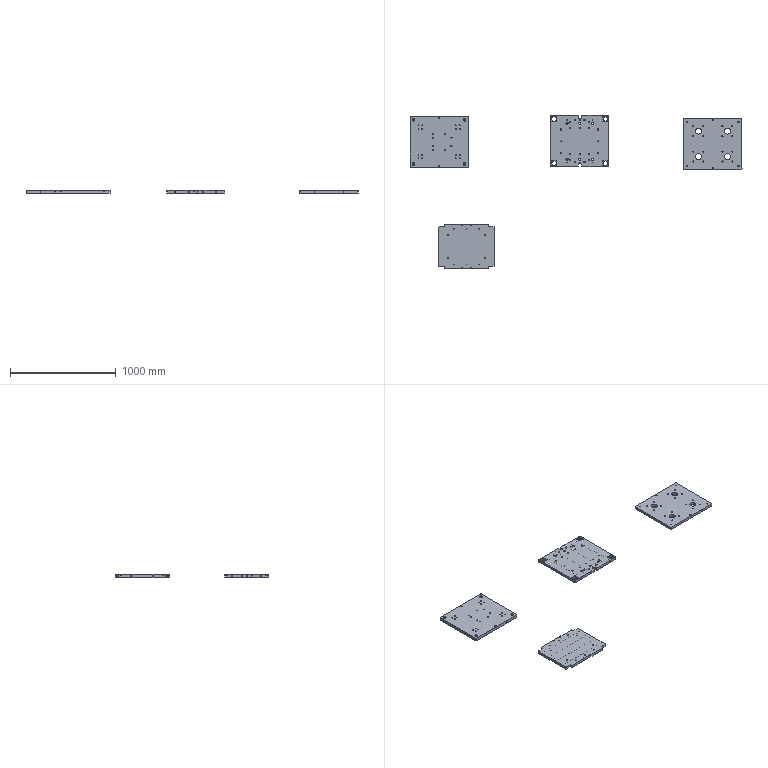NC program | Mastercam | posted with a generic post | part box 3140 x 1452 x 30 mm
Lines 4752 to 6153 of 6493, first 1239 of 1402 lines:
N7860 T7 M6
N7870 G0 G90 G17 G54 X-230.95 Y208.6 A0. S6000 M3
N7880 G43 H7 Z50. M8
N7890 Z1.2
N7900 G1 Z-.75 F600.
N7910 X-230.55 F1000.
N7920 G3 X-230.15 Y209. I0. J.4
N7930 X-242. Y220.85 I-11.85 J0.
N7940 X-253.85 Y209. I0. J-11.85
N7950 X-242. Y197.15 I11.85 J0.
N7960 X-230.15 Y209. I0. J11.85
N7970 X-230.161 Y209.5 I-11.85 J0.
N7980 X-230.56 Y209.882 I-.399 J-.017
N7990 X-230.577 Y209.883 I0. J-.399
N8000 G1 X-230.977 Y209.866
N8010 G0 Z50.
N8020 X-237.95 Y208.6
N8030 Z-11.8
N8040 G1 Z-13.75 F600.
N8050 X-237.55 F1000.
N8060 G3 X-237.15 Y209. I0. J.4
N8070 X-242. Y213.85 I-4.85 J0.
N8080 X-246.85 Y209. I0. J-4.85
N8090 X-242. Y204.15 I4.85 J0.
N8100 X-237.15 Y209. I0. J4.85
N8110 X-237.176 Y209.499 I-4.85 J0.
N8120 X-237.574 Y209.858 I-.398 J-.041
N8130 X-237.615 Y209.856 I0. J-.4
N8140 G1 X-238.013 Y209.815
N8150 G0 Z50.
N8160 X4.05 Y227.1
N8170 Z1.2
N8180 G1 Z-.75 F600.
N8190 X4.45 F1000.
N8200 G3 X4.85 Y227.5 I0. J.4
N8210 X0. Y232.35 I-4.85 J0.
N8220 X-4.85 Y227.5 I0. J-4.85
N8230 X0. Y222.65 I4.85 J0.
N8240 X4.85 Y227.5 I0. J4.85
N8250 X4.824 Y227.999 I-4.85 J0.
N8260 X4.426 Y228.358 I-.398 J-.041
N8270 X4.385 Y228.356 I0. J-.4
N8280 G1 X3.987 Y228.315
N8290 G0 Z50.
N8300 X253.05 Y208.6
N8310 Z1.2
N8320 G1 Z-.75 F600.
N8330 X253.45 F1000.
N8340 G3 X253.85 Y209. I0. J.4
N8350 X242. Y220.85 I-11.85 J0.
N8360 X230.15 Y209. I0. J-11.85
N8370 X242. Y197.15 I11.85 J0.
N8380 X253.85 Y209. I0. J11.85
N8390 X253.839 Y209.5 I-11.85 J0.
N8400 X253.44 Y209.882 I-.399 J-.017
N8410 X253.423 Y209.883 I0. J-.399
N8420 G1 X253.023 Y209.866
N8430 G0 Z50.
N8440 X246.05 Y208.6
N8450 Z-11.8
N8460 G1 Z-13.75 F600.
N8470 X246.45 F1000.
N8480 G3 X246.85 Y209. I0. J.4
N8490 X242. Y213.85 I-4.85 J0.
N8500 X237.15 Y209. I0. J-4.85
N8510 X242. Y204.15 I4.85 J0.
N8520 X246.85 Y209. I0. J4.85
N8530 X246.824 Y209.499 I-4.85 J0.
N8540 X246.426 Y209.858 I-.398 J-.041
N8550 X246.385 Y209.856 I0. J-.4
N8560 G1 X245.987 Y209.815
N8570 G0 Z50.
N8580 X197.55 Y155.6
N8590 Z1.2
N8600 G1 Z-.75 F600.
N8610 X197.95 F1000.
N8620 G3 X198.35 Y156. I0. J.4
N8630 X194.5 Y159.85 I-3.85 J0.
N8640 X190.65 Y156. I0. J-3.85
N8650 X194.5 Y152.15 I3.85 J0.
N8660 X198.35 Y156. I0. J3.85
N8670 X198.318 Y156.499 I-3.85 J0.
N8680 X197.921 Y156.847 I-.397 J-.052
N8690 X197.869 Y156.843 I0. J-.4
N8700 G1 X197.473 Y156.792
N8710 G0 Z50.
N8720 X161.55 Y155.6
N8730 Z1.2
N8740 G1 Z-.75 F600.
N8750 X161.95 F1000.
N8760 G3 X162.35 Y156. I0. J.4
N8770 X158.5 Y159.85 I-3.85 J0.
N8780 X154.65 Y156. I0. J-3.85
N8790 X158.5 Y152.15 I3.85 J0.
N8800 X162.35 Y156. I0. J3.85
N8810 X162.318 Y156.499 I-3.85 J0.
N8820 X161.921 Y156.847 I-.397 J-.052
N8830 X161.869 Y156.843 I0. J-.4
N8840 G1 X161.473 Y156.792
N8850 G0 Z50.
N8860 X161.55 Y123.6
N8870 Z1.2
N8880 G1 Z-.75 F600.
N8890 X161.95 F1000.
N8900 G3 X162.35 Y124. I0. J.4
N8910 X158.5 Y127.85 I-3.85 J0.
N8920 X154.65 Y124. I0. J-3.85
N8930 X158.5 Y120.15 I3.85 J0.
N8940 X162.35 Y124. I0. J3.85
N8950 X162.318 Y124.499 I-3.85 J0.
N8960 X161.921 Y124.847 I-.397 J-.052
N8970 X161.869 Y124.843 I0. J-.4
N8980 G1 X161.473 Y124.792
N8990 G0 Z50.
N9000 X197.55 Y123.6
N9010 Z1.2
N9020 G1 Z-.75 F600.
N9030 X197.95 F1000.
N9040 G3 X198.35 Y124. I0. J.4
N9050 X194.5 Y127.85 I-3.85 J0.
N9060 X190.65 Y124. I0. J-3.85
N9070 X194.5 Y120.15 I3.85 J0.
N9080 X198.35 Y124. I0. J3.85
N9090 X198.318 Y124.499 I-3.85 J0.
N9100 X197.921 Y124.847 I-.397 J-.052
N9110 X197.869 Y124.843 I0. J-.4
N9120 G1 X197.473 Y124.792
N9130 G0 Z50.
N9140 X-155.45 Y155.6
N9150 Z1.2
N9160 G1 Z-.75 F600.
N9170 X-155.05 F1000.
N9180 G3 X-154.65 Y156. I0. J.4
N9190 X-158.5 Y159.85 I-3.85 J0.
N9200 X-162.35 Y156. I0. J-3.85
N9210 X-158.5 Y152.15 I3.85 J0.
N9220 X-154.65 Y156. I0. J3.85
N9230 X-154.682 Y156.499 I-3.85 J0.
N9240 X-155.079 Y156.847 I-.397 J-.052
N9250 X-155.131 Y156.843 I0. J-.4
N9260 G1 X-155.527 Y156.792
N9270 G0 Z50.
N9280 X-191.45 Y155.6
N9290 Z1.2
N9300 G1 Z-.75 F600.
N9310 X-191.05 F1000.
N9320 G3 X-190.65 Y156. I0. J.4
N9330 X-194.5 Y159.85 I-3.85 J0.
N9340 X-198.35 Y156. I0. J-3.85
N9350 X-194.5 Y152.15 I3.85 J0.
N9360 X-190.65 Y156. I0. J3.85
N9370 X-190.682 Y156.499 I-3.85 J0.
N9380 X-191.079 Y156.847 I-.397 J-.052
N9390 X-191.131 Y156.843 I0. J-.4
N9400 G1 X-191.527 Y156.792
N9410 G0 Z50.
N9420 X-191.45 Y123.6
N9430 Z1.2
N9440 G1 Z-.75 F600.
N9450 X-191.05 F1000.
N9460 G3 X-190.65 Y124. I0. J.4
N9470 X-194.5 Y127.85 I-3.85 J0.
N9480 X-198.35 Y124. I0. J-3.85
N9490 X-194.5 Y120.15 I3.85 J0.
N9500 X-190.65 Y124. I0. J3.85
N9510 X-190.682 Y124.499 I-3.85 J0.
N9520 X-191.079 Y124.847 I-.397 J-.052
N9530 X-191.131 Y124.843 I0. J-.4
N9540 G1 X-191.527 Y124.792
N9550 G0 Z50.
N9560 X-155.45 Y123.6
N9570 Z1.2
N9580 G1 Z-.75 F600.
N9590 X-155.05 F1000.
N9600 G3 X-154.65 Y124. I0. J.4
N9610 X-158.5 Y127.85 I-3.85 J0.
N9620 X-162.35 Y124. I0. J-3.85
N9630 X-158.5 Y120.15 I3.85 J0.
N9640 X-154.65 Y124. I0. J3.85
N9650 X-154.682 Y124.499 I-3.85 J0.
N9660 X-155.079 Y124.847 I-.397 J-.052
N9670 X-155.131 Y124.843 I0. J-.4
N9680 G1 X-155.527 Y124.792
N9690 G0 Z50.
N9700 X-51.2 Y72.1
N9710 Z1.2
N9720 G1 Z-.75 F600.
N9730 X-50.8 F1000.
N9740 G3 X-50.4 Y72.5 I0. J.4
N9750 X-55. Y77.1 I-4.6 J0.
N9760 X-59.6 Y72.5 I0. J-4.6
N9770 X-55. Y67.9 I4.6 J0.
N9780 X-50.4 Y72.5 I0. J4.6
N9790 X-50.427 Y72.999 I-4.6 J0.
N9800 X-50.825 Y73.356 I-.398 J-.043
N9810 X-50.868 Y73.353 I0. J-.4
N9820 G1 X-51.266 Y73.31
N9830 G0 Z50.
N9840 X58.8 Y72.1
N9850 Z1.2
N9860 G1 Z-.75 F600.
N9870 X59.2 F1000.
N9880 G3 X59.6 Y72.5 I0. J.4
N9890 X55. Y77.1 I-4.6 J0.
N9900 X50.4 Y72.5 I0. J-4.6
N9910 X55. Y67.9 I4.6 J0.
N9920 X59.6 Y72.5 I0. J4.6
N9930 X59.573 Y72.999 I-4.6 J0.
N9940 X59.175 Y73.356 I-.398 J-.043
N9950 X59.132 Y73.353 I0. J-.4
N9960 G1 X58.734 Y73.31
N9970 G0 Z50.
N9980 X120.8 Y39.6
N9990 Z1.2
N100 G1 Z-.75 F600.
N110 X121.2 F1000.
N120 G3 X121.6 Y40. I0. J.4
N130 X117. Y44.6 I-4.6 J0.
N140 X112.4 Y40. I0. J-4.6
N150 X117. Y35.4 I4.6 J0.
N160 X121.6 Y40. I0. J4.6
N170 X121.573 Y40.499 I-4.6 J0.
N180 X121.175 Y40.856 I-.398 J-.043
N190 X121.132 Y40.853 I0. J-.4
N200 G1 X120.734 Y40.81
N210 G0 Z50.
N220 X120.8 Y-40.4
N230 Z1.2
N240 G1 Z-.75 F600.
N250 X121.2 F1000.
N260 G3 X121.6 Y-40. I0. J.4
N270 X117. Y-35.4 I-4.6 J0.
N280 X112.4 Y-40. I0. J-4.6
N290 X117. Y-44.6 I4.6 J0.
N300 X121.6 Y-40. I0. J4.6
N310 X121.573 Y-39.501 I-4.6 J0.
N320 X121.175 Y-39.144 I-.398 J-.043
N330 X121.132 Y-39.147 I0. J-.4
N340 G1 X120.734 Y-39.19
N350 G0 Z50.
N360 X58.8 Y-72.9
N370 Z1.2
N380 G1 Z-.75 F600.
N390 X59.2 F1000.
N400 G3 X59.6 Y-72.5 I0. J.4
N410 X55. Y-67.9 I-4.6 J0.
N420 X50.4 Y-72.5 I0. J-4.6
N430 X55. Y-77.1 I4.6 J0.
N440 X59.6 Y-72.5 I0. J4.6
N450 X59.573 Y-72.001 I-4.6 J0.
N460 X59.175 Y-71.644 I-.398 J-.043
N470 X59.132 Y-71.647 I0. J-.4
N480 G1 X58.734 Y-71.69
N490 G0 Z50.
N500 X161.55 Y-124.4
N510 Z1.2
N520 G1 Z-.75 F600.
N530 X161.95 F1000.
N540 G3 X162.35 Y-124. I0. J.4
N550 X158.5 Y-120.15 I-3.85 J0.
N560 X154.65 Y-124. I0. J-3.85
N570 X158.5 Y-127.85 I3.85 J0.
N580 X162.35 Y-124. I0. J3.85
N590 X162.318 Y-123.501 I-3.85 J0.
N600 X161.921 Y-123.153 I-.397 J-.052
N610 X161.869 Y-123.157 I0. J-.4
N620 G1 X161.473 Y-123.208
N630 G0 Z50.
N640 X197.55 Y-124.4
N650 Z1.2
N660 G1 Z-.75 F600.
N670 X197.95 F1000.
N680 G3 X198.35 Y-124. I0. J.4
N690 X194.5 Y-120.15 I-3.85 J0.
N700 X190.65 Y-124. I0. J-3.85
N710 X194.5 Y-127.85 I3.85 J0.
N720 X198.35 Y-124. I0. J3.85
N730 X198.318 Y-123.501 I-3.85 J0.
N740 X197.921 Y-123.153 I-.397 J-.052
N750 X197.869 Y-123.157 I0. J-.4
N760 G1 X197.473 Y-123.208
N770 G0 Z50.
N780 X197.55 Y-156.4
N790 Z1.2
N800 G1 Z-.75 F600.
N810 X197.95 F1000.
N820 G3 X198.35 Y-156. I0. J.4
N830 X194.5 Y-152.15 I-3.85 J0.
N840 X190.65 Y-156. I0. J-3.85
N850 X194.5 Y-159.85 I3.85 J0.
N860 X198.35 Y-156. I0. J3.85
N870 X198.318 Y-155.501 I-3.85 J0.
N880 X197.921 Y-155.153 I-.397 J-.052
N890 X197.869 Y-155.157 I0. J-.4
N900 G1 X197.473 Y-155.208
N910 G0 Z50.
N920 X161.55 Y-156.4
N930 Z1.2
N940 G1 Z-.75 F600.
N950 X161.95 F1000.
N960 G3 X162.35 Y-156. I0. J.4
N970 X158.5 Y-152.15 I-3.85 J0.
N980 X154.65 Y-156. I0. J-3.85
N990 X158.5 Y-159.85 I3.85 J0.
N1000 X162.35 Y-156. I0. J3.85
N1010 X162.318 Y-155.501 I-3.85 J0.
N1020 X161.921 Y-155.153 I-.397 J-.052
N1030 X161.869 Y-155.157 I0. J-.4
N1040 G1 X161.473 Y-155.208
N1050 G0 Z50.
N1060 X253.05 Y-209.4
N1070 Z1.2
N1080 G1 Z-.75 F600.
N1090 X253.45 F1000.
N1100 G3 X253.85 Y-209. I0. J.4
N1110 X242. Y-197.15 I-11.85 J0.
N1120 X230.15 Y-209. I0. J-11.85
N1130 X242. Y-220.85 I11.85 J0.
N1140 X253.85 Y-209. I0. J11.85
N1150 X253.839 Y-208.5 I-11.85 J0.
N1160 X253.44 Y-208.118 I-.399 J-.017
N1170 X253.423 Y-208.117 I0. J-.399
N1180 G1 X253.023 Y-208.134
N1190 G0 Z50.
N1200 X246.05 Y-209.4
N1210 Z-11.8
N1220 G1 Z-13.75 F600.
N1230 X246.45 F1000.
N1240 G3 X246.85 Y-209. I0. J.4
N1250 X242. Y-204.15 I-4.85 J0.
N1260 X237.15 Y-209. I0. J-4.85
N1270 X242. Y-213.85 I4.85 J0.
N1280 X246.85 Y-209. I0. J4.85
N1290 X246.824 Y-208.501 I-4.85 J0.
N1300 X246.426 Y-208.142 I-.398 J-.041
N1310 X246.385 Y-208.144 I0. J-.4
N1320 G1 X245.987 Y-208.185
N1330 G0 Z50.
N1340 X4.05 Y-227.9
N1350 Z1.2
N1360 G1 Z-.75 F600.
N1370 X4.45 F1000.
N1380 G3 X4.85 Y-227.5 I0. J.4
N1390 X0. Y-222.65 I-4.85 J0.
N1400 X-4.85 Y-227.5 I0. J-4.85
N1410 X0. Y-232.35 I4.85 J0.
N1420 X4.85 Y-227.5 I0. J4.85
N1430 X4.824 Y-227.001 I-4.85 J0.
N1440 X4.426 Y-226.642 I-.398 J-.041
N1450 X4.385 Y-226.644 I0. J-.4
N1460 G1 X3.987 Y-226.685
N1470 G0 Z50.
N1480 X-51.2 Y-72.9
N1490 Z1.2
N1500 G1 Z-.75 F600.
N1510 X-50.8 F1000.
N1520 G3 X-50.4 Y-72.5 I0. J.4
N1530 X-55. Y-67.9 I-4.6 J0.
N1540 X-59.6 Y-72.5 I0. J-4.6
N1550 X-55. Y-77.1 I4.6 J0.
N1560 X-50.4 Y-72.5 I0. J4.6
N1570 X-50.427 Y-72.001 I-4.6 J0.
N1580 X-50.825 Y-71.644 I-.398 J-.043
N1590 X-50.868 Y-71.647 I0. J-.4
N1600 G1 X-51.266 Y-71.69
N1610 G0 Z50.
N1620 X-53.2 Y-40.4
N1630 Z1.2
N1640 G1 Z-.75 F600.
N1650 X-52.8 F1000.
N1660 G3 X-52.4 Y-40. I0. J.4
N1670 X-57. Y-35.4 I-4.6 J0.
N1680 X-61.6 Y-40. I0. J-4.6
N1690 X-57. Y-44.6 I4.6 J0.
N1700 X-52.4 Y-40. I0. J4.6
N1710 X-52.427 Y-39.501 I-4.6 J0.
N1720 X-52.825 Y-39.144 I-.398 J-.043
N1730 X-52.868 Y-39.147 I0. J-.4
N1740 G1 X-53.266 Y-39.19
N1750 G0 Z50.
N1760 X-53.2 Y39.6
N1770 Z1.2
N1780 G1 Z-.75 F600.
N1790 X-52.8 F1000.
N1800 G3 X-52.4 Y40. I0. J.4
N1810 X-57. Y44.6 I-4.6 J0.
N1820 X-61.6 Y40. I0. J-4.6
N1830 X-57. Y35.4 I4.6 J0.
N1840 X-52.4 Y40. I0. J4.6
N1850 X-52.427 Y40.499 I-4.6 J0.
N1860 X-52.825 Y40.856 I-.398 J-.043
N1870 X-52.868 Y40.853 I0. J-.4
N1880 G1 X-53.266 Y40.81
N1890 G0 Z50.
N1900 X-155.45 Y-124.4
N1910 Z1.2
N1920 G1 Z-.75 F600.
N1930 X-155.05 F1000.
N1940 G3 X-154.65 Y-124. I0. J.4
N1950 X-158.5 Y-120.15 I-3.85 J0.
N1960 X-162.35 Y-124. I0. J-3.85
N1970 X-158.5 Y-127.85 I3.85 J0.
N1980 X-154.65 Y-124. I0. J3.85
N1990 X-154.682 Y-123.501 I-3.85 J0.
N2000 X-155.079 Y-123.153 I-.397 J-.052
N2010 X-155.131 Y-123.157 I0. J-.4
N2020 G1 X-155.527 Y-123.208
N2030 G0 Z50.
N2040 X-191.45 Y-124.4
N2050 Z1.2
N2060 G1 Z-.75 F600.
N2070 X-191.05 F1000.
N2080 G3 X-190.65 Y-124. I0. J.4
N2090 X-194.5 Y-120.15 I-3.85 J0.
N2100 X-198.35 Y-124. I0. J-3.85
N2110 X-194.5 Y-127.85 I3.85 J0.
N2120 X-190.65 Y-124. I0. J3.85
N2130 X-190.682 Y-123.501 I-3.85 J0.
N2140 X-191.079 Y-123.153 I-.397 J-.052
N2150 X-191.131 Y-123.157 I0. J-.4
N2160 G1 X-191.527 Y-123.208
N2170 G0 Z50.
N2180 X-191.45 Y-156.4
N2190 Z1.2
N2200 G1 Z-.75 F600.
N2210 X-191.05 F1000.
N2220 G3 X-190.65 Y-156. I0. J.4
N2230 X-194.5 Y-152.15 I-3.85 J0.
N2240 X-198.35 Y-156. I0. J-3.85
N2250 X-194.5 Y-159.85 I3.85 J0.
N2260 X-190.65 Y-156. I0. J3.85
N2270 X-190.682 Y-155.501 I-3.85 J0.
N2280 X-191.079 Y-155.153 I-.397 J-.052
N2290 X-191.131 Y-155.157 I0. J-.4
N2300 G1 X-191.527 Y-155.208
N2310 G0 Z50.
N2320 X-155.45 Y-156.4
N2330 Z1.2
N2340 G1 Z-.75 F600.
N2350 X-155.05 F1000.
N2360 G3 X-154.65 Y-156. I0. J.4
N2370 X-158.5 Y-152.15 I-3.85 J0.
N2380 X-162.35 Y-156. I0. J-3.85
N2390 X-158.5 Y-159.85 I3.85 J0.
N2400 X-154.65 Y-156. I0. J3.85
N2410 X-154.682 Y-155.501 I-3.85 J0.
N2420 X-155.079 Y-155.153 I-.397 J-.052
N2430 X-155.131 Y-155.157 I0. J-.4
N2440 G1 X-155.527 Y-155.208
N2450 G0 Z50.
N2460 X-230.95 Y-209.4
N2470 Z1.2
N2480 G1 Z-.75 F600.
N2490 X-230.55 F1000.
N2500 G3 X-230.15 Y-209. I0. J.4
N2510 X-242. Y-197.15 I-11.85 J0.
N2520 X-253.85 Y-209. I0. J-11.85
N2530 X-242. Y-220.85 I11.85 J0.
N2540 X-230.15 Y-209. I0. J11.85
N2550 X-230.161 Y-208.5 I-11.85 J0.
N2560 X-230.56 Y-208.118 I-.399 J-.017
N2570 X-230.577 Y-208.117 I0. J-.399
N2580 G1 X-230.977 Y-208.134
N2590 G0 Z50.
N2600 X-237.95 Y-209.4
N2610 Z-11.8
N2620 G1 Z-13.75 F600.
N2630 X-237.55 F1000.
N2640 G3 X-237.15 Y-209. I0. J.4
N2650 X-242. Y-204.15 I-4.85 J0.
N2660 X-246.85 Y-209. I0. J-4.85
N2670 X-242. Y-213.85 I4.85 J0.
N2680 X-237.15 Y-209. I0. J4.85
N2690 X-237.176 Y-208.501 I-4.85 J0.
N2700 X-237.574 Y-208.142 I-.398 J-.041
N2710 X-237.615 Y-208.144 I0. J-.4
N2720 G1 X-238.013 Y-208.185
N2730 G0 Z50.
N2740 X-193.7 Y-156.4
N2750 Z-12.8
N2760 G1 Z-15.25 F600.
N2770 X-193.3 F1000.
N2780 G3 X-192.9 Y-156. I0. J.4
N2790 X-194.5 Y-154.4 I-1.6 J0.
N2800 X-196.1 Y-156. I0. J-1.6
N2810 X-194.5 Y-157.6 I1.6 J0.
N2820 X-192.9 Y-156. I0. J1.6
N2830 X-192.977 Y-155.508 I-1.6 J0.
N2840 X-193.358 Y-155.231 I-.381 J-.123
N2850 X-193.481 Y-155.25 I0. J-.4
N2860 G1 X-193.862 Y-155.373
N2870 G0 Z50.
N2880 X-193.7 Y-124.4
N2890 Z-12.8
N2900 G1 Z-15.25 F600.
N2910 X-193.3 F1000.
N2920 G3 X-192.9 Y-124. I0. J.4
N2930 X-194.5 Y-122.4 I-1.6 J0.
N2940 X-196.1 Y-124. I0. J-1.6
N2950 X-194.5 Y-125.6 I1.6 J0.
N2960 X-192.9 Y-124. I0. J1.6
N2970 X-192.977 Y-123.508 I-1.6 J0.
N2980 X-193.358 Y-123.231 I-.381 J-.123
N2990 X-193.481 Y-123.25 I0. J-.4
N3000 G1 X-193.862 Y-123.373
N3010 G0 Z50.
N3020 X-157.7 Y-124.4
N3030 Z-12.8
N3040 G1 Z-15.25 F600.
N3050 X-157.3 F1000.
N3060 G3 X-156.9 Y-124. I0. J.4
N3070 X-158.5 Y-122.4 I-1.6 J0.
N3080 X-160.1 Y-124. I0. J-1.6
N3090 X-158.5 Y-125.6 I1.6 J0.
N3100 X-156.9 Y-124. I0. J1.6
N3110 X-156.977 Y-123.508 I-1.6 J0.
N3120 X-157.358 Y-123.231 I-.381 J-.123
N3130 X-157.481 Y-123.25 I0. J-.4
N3140 G1 X-157.862 Y-123.373
N3150 G0 Z50.
N3160 X-157.7 Y-156.4
N3170 Z-12.8
N3180 G1 Z-15.25 F600.
N3190 X-157.3 F1000.
N3200 G3 X-156.9 Y-156. I0. J.4
N3210 X-158.5 Y-154.4 I-1.6 J0.
N3220 X-160.1 Y-156. I0. J-1.6
N3230 X-158.5 Y-157.6 I1.6 J0.
N3240 X-156.9 Y-156. I0. J1.6
N3250 X-156.977 Y-155.508 I-1.6 J0.
N3260 X-157.358 Y-155.231 I-.381 J-.123
N3270 X-157.481 Y-155.25 I0. J-.4
N3280 G1 X-157.862 Y-155.373
N3290 G0 Z50.
N3300 X159.3 Y-124.4
N3310 Z-12.8
N3320 G1 Z-15.25 F600.
N3330 X159.7 F1000.
N3340 G3 X160.1 Y-124. I0. J.4
N3350 X158.5 Y-122.4 I-1.6 J0.
N3360 X156.9 Y-124. I0. J-1.6
N3370 X158.5 Y-125.6 I1.6 J0.
N3380 X160.1 Y-124. I0. J1.6
N3390 X160.023 Y-123.508 I-1.6 J0.
N3400 X159.642 Y-123.231 I-.381 J-.123
N3410 X159.519 Y-123.25 I0. J-.4
N3420 G1 X159.138 Y-123.373
N3430 G0 Z50.
N3440 X159.3 Y-156.4
N3450 Z-12.8
N3460 G1 Z-15.25 F600.
N3470 X159.7 F1000.
N3480 G3 X160.1 Y-156. I0. J.4
N3490 X158.5 Y-154.4 I-1.6 J0.
N3500 X156.9 Y-156. I0. J-1.6
N3510 X158.5 Y-157.6 I1.6 J0.
N3520 X160.1 Y-156. I0. J1.6
N3530 X160.023 Y-155.508 I-1.6 J0.
N3540 X159.642 Y-155.231 I-.381 J-.123
N3550 X159.519 Y-155.25 I0. J-.4
N3560 G1 X159.138 Y-155.373
N3570 G0 Z50.
N3580 X195.3 Y-156.4
N3590 Z-12.8
N3600 G1 Z-15.25 F600.
N3610 X195.7 F1000.
N3620 G3 X196.1 Y-156. I0. J.4
N3630 X194.5 Y-154.4 I-1.6 J0.
N3640 X192.9 Y-156. I0. J-1.6
N3650 X194.5 Y-157.6 I1.6 J0.
N3660 X196.1 Y-156. I0. J1.6
N3670 X196.023 Y-155.508 I-1.6 J0.
N3680 X195.642 Y-155.231 I-.381 J-.123
N3690 X195.519 Y-155.25 I0. J-.4
N3700 G1 X195.138 Y-155.373
N3710 G0 Z50.
N3720 X195.3 Y-124.4
N3730 Z-12.8
N3740 G1 Z-15.25 F600.
N3750 X195.7 F1000.
N3760 G3 X196.1 Y-124. I0. J.4
N3770 X194.5 Y-122.4 I-1.6 J0.
N3780 X192.9 Y-124. I0. J-1.6
N3790 X194.5 Y-125.6 I1.6 J0.
N3800 X196.1 Y-124. I0. J1.6
N3810 X196.023 Y-123.508 I-1.6 J0.
N3820 X195.642 Y-123.231 I-.381 J-.123
N3830 X195.519 Y-123.25 I0. J-.4
N3840 G1 X195.138 Y-123.373
N3850 G0 Z50.
N3860 X195.3 Y123.6
N3870 Z-12.8
N3880 G1 Z-15.25 F600.
N3890 X195.7 F1000.
N3900 G3 X196.1 Y124. I0. J.4
N3910 X194.5 Y125.6 I-1.6 J0.
N3920 X192.9 Y124. I0. J-1.6
N3930 X194.5 Y122.4 I1.6 J0.
N3940 X196.1 Y124. I0. J1.6
N3950 X196.023 Y124.492 I-1.6 J0.
N3960 X195.642 Y124.769 I-.381 J-.123
N3970 X195.519 Y124.75 I0. J-.4
N3980 G1 X195.138 Y124.627
N3990 G0 Z50.
N4000 X159.3 Y123.6
N4010 Z-12.8
N4020 G1 Z-15.25 F600.
N4030 X159.7 F1000.
N4040 G3 X160.1 Y124. I0. J.4
N4050 X158.5 Y125.6 I-1.6 J0.
N4060 X156.9 Y124. I0. J-1.6
N4070 X158.5 Y122.4 I1.6 J0.
N4080 X160.1 Y124. I0. J1.6
N4090 X160.023 Y124.492 I-1.6 J0.
N4100 X159.642 Y124.769 I-.381 J-.123
N4110 X159.519 Y124.75 I0. J-.4
N4120 G1 X159.138 Y124.627
N4130 G0 Z50.
N4140 X159.3 Y155.6
N4150 Z-12.8
N4160 G1 Z-15.25 F600.
N4170 X159.7 F1000.
N4180 G3 X160.1 Y156. I0. J.4
N4190 X158.5 Y157.6 I-1.6 J0.
N4200 X156.9 Y156. I0. J-1.6
N4210 X158.5 Y154.4 I1.6 J0.
N4220 X160.1 Y156. I0. J1.6
N4230 X160.023 Y156.492 I-1.6 J0.
N4240 X159.642 Y156.769 I-.381 J-.123
N4250 X159.519 Y156.75 I0. J-.4
N4260 G1 X159.138 Y156.627
N4270 G0 Z50.
N4280 X195.3 Y155.6
N4290 Z-12.8
N4300 G1 Z-15.25 F600.
N4310 X195.7 F1000.
N4320 G3 X196.1 Y156. I0. J.4
N4330 X194.5 Y157.6 I-1.6 J0.
N4340 X192.9 Y156. I0. J-1.6
N4350 X194.5 Y154.4 I1.6 J0.
N4360 X196.1 Y156. I0. J1.6
N4370 X196.023 Y156.492 I-1.6 J0.
N4380 X195.642 Y156.769 I-.381 J-.123
N4390 X195.519 Y156.75 I0. J-.4
N4400 G1 X195.138 Y156.627
N4410 G0 Z50.
N4420 X-157.7 Y123.6
N4430 Z-12.8
N4440 G1 Z-15.25 F600.
N4450 X-157.3 F1000.
N4460 G3 X-156.9 Y124. I0. J.4
N4470 X-158.5 Y125.6 I-1.6 J0.
N4480 X-160.1 Y124. I0. J-1.6
N4490 X-158.5 Y122.4 I1.6 J0.
N4500 X-156.9 Y124. I0. J1.6
N4510 X-156.977 Y124.492 I-1.6 J0.
N4520 X-157.358 Y124.769 I-.381 J-.123
N4530 X-157.481 Y124.75 I0. J-.4
N4540 G1 X-157.862 Y124.627
N4550 G0 Z50.
N4560 X-157.7 Y155.6
N4570 Z-12.8
N4580 G1 Z-15.25 F600.
N4590 X-157.3 F1000.
N4600 G3 X-156.9 Y156. I0. J.4
N4610 X-158.5 Y157.6 I-1.6 J0.
N4620 X-160.1 Y156. I0. J-1.6
N4630 X-158.5 Y154.4 I1.6 J0.
N4640 X-156.9 Y156. I0. J1.6
N4650 X-156.977 Y156.492 I-1.6 J0.
N4660 X-157.358 Y156.769 I-.381 J-.123
N4670 X-157.481 Y156.75 I0. J-.4
N4680 G1 X-157.862 Y156.627
N4690 G0 Z50.
N4700 X-193.7 Y155.6
N4710 Z-12.8
N4720 G1 Z-15.25 F600.
N4730 X-193.3 F1000.
N4740 G3 X-192.9 Y156. I0. J.4
N4750 X-194.5 Y157.6 I-1.6 J0.
N4760 X-196.1 Y156. I0. J-1.6
N4770 X-194.5 Y154.4 I1.6 J0.
N4780 X-192.9 Y156. I0. J1.6
N4790 X-192.977 Y156.492 I-1.6 J0.
N4800 X-193.358 Y156.769 I-.381 J-.123
N4810 X-193.481 Y156.75 I0. J-.4
N4820 G1 X-193.862 Y156.627
N4830 G0 Z50.
N4840 X-193.7 Y123.6
N4850 Z-12.8
N4860 G1 Z-15.25 F600.
N4870 X-193.3 F1000.
N4880 G3 X-192.9 Y124. I0. J.4
N4890 X-194.5 Y125.6 I-1.6 J0.
N4900 X-196.1 Y124. I0. J-1.6
N4910 X-194.5 Y122.4 I1.6 J0.
N4920 X-192.9 Y124. I0. J1.6
N4930 X-192.977 Y124.492 I-1.6 J0.
N4940 X-193.358 Y124.769 I-.381 J-.123
N4950 X-193.481 Y124.75 I0. J-.4
N4960 G1 X-193.862 Y124.627
N4970 G0 Z50.
N4980 M5
N4990 G91 G28 Z0. M9
N5000 A0.
N5010 M01
N5020 T8 M6
N5030 G0 G90 G17 G54 X-245.93 Y209. A0. S7000 M3
N5040 G43 H8 Z50. M8
N5050 Z1.5
N5060 G1 Z.5 F600.
N5070 G3 X-242. Y205.07 Z.375 I3.93 J0. F2000.
N5080 X-238.07 Y209. Z.25 I0. J3.93
N5090 X-242. Y212.93 Z.125 I-3.93 J0.
N5100 X-245.93 Y209. Z0. I0. J-3.93
N5110 X-242. Y205.07 Z-.125 I3.93 J0.
N5120 X-238.07 Y209. Z-.25 I0. J3.93
N5130 X-242. Y212.93 Z-.375 I-3.93 J0.
N5140 X-245.93 Y209. Z-.5 I0. J-3.93
N5150 X-242. Y205.07 Z-.625 I3.93 J0.
N5160 X-238.07 Y209. Z-.75 I0. J3.93
N5170 X-242. Y212.93 Z-.875 I-3.93 J0.
N5180 X-245.93 Y209. Z-1. I0. J-3.93
N5190 X-242. Y205.07 Z-1.125 I3.93 J0.
N5200 X-238.07 Y209. Z-1.25 I0. J3.93
N5210 X-242. Y212.93 Z-1.375 I-3.93 J0.
N5220 X-245.93 Y209. Z-1.5 I0. J-3.93
N5230 X-242. Y205.07 Z-1.625 I3.93 J0.
N5240 X-238.07 Y209. Z-1.75 I0. J3.93
N5250 X-242. Y212.93 Z-1.875 I-3.93 J0.
N5260 X-245.93 Y209. Z-2. I0. J-3.93
N5270 X-242. Y205.07 Z-2.125 I3.93 J0.
N5280 X-238.07 Y209. Z-2.25 I0. J3.93
N5290 X-242. Y212.93 Z-2.375 I-3.93 J0.
N5300 X-245.93 Y209. Z-2.5 I0. J-3.93
N5310 X-242. Y205.07 Z-2.625 I3.93 J0.
N5320 X-238.07 Y209. Z-2.75 I0. J3.93
N5330 X-242. Y212.93 Z-2.875 I-3.93 J0.
N5340 X-245.93 Y209. Z-3. I0. J-3.93
N5350 X-242. Y205.07 Z-3.125 I3.93 J0.
N5360 X-238.07 Y209. Z-3.25 I0. J3.93
N5370 X-242. Y212.93 Z-3.375 I-3.93 J0.
N5380 X-245.93 Y209. Z-3.5 I0. J-3.93
N5390 X-242. Y205.07 Z-3.625 I3.93 J0.
N5400 X-238.07 Y209. Z-3.75 I0. J3.93
N5410 X-242. Y212.93 Z-3.875 I-3.93 J0.
N5420 X-245.93 Y209. Z-4. I0. J-3.93
N5430 X-242. Y205.07 Z-4.125 I3.93 J0.
N5440 X-238.07 Y209. Z-4.25 I0. J3.93
N5450 X-242. Y212.93 Z-4.375 I-3.93 J0.
N5460 X-245.93 Y209. Z-4.5 I0. J-3.93
N5470 X-242. Y205.07 Z-4.625 I3.93 J0.
N5480 X-238.07 Y209. Z-4.75 I0. J3.93
N5490 X-242. Y212.93 Z-4.875 I-3.93 J0.
N5500 X-245.93 Y209. Z-5. I0. J-3.93
N5510 X-242. Y205.07 Z-5.125 I3.93 J0.
N5520 X-238.07 Y209. Z-5.25 I0. J3.93
N5530 X-242. Y212.93 Z-5.375 I-3.93 J0.
N5540 X-245.93 Y209. Z-5.5 I0. J-3.93
N5550 X-242. Y205.07 Z-5.625 I3.93 J0.
N5560 X-238.07 Y209. Z-5.75 I0. J3.93
N5570 X-242. Y212.93 Z-5.875 I-3.93 J0.
N5580 X-245.93 Y209. Z-6. I0. J-3.93
N5590 X-242. Y205.07 Z-6.125 I3.93 J0.
N5600 X-238.07 Y209. Z-6.25 I0. J3.93
N5610 X-242. Y212.93 Z-6.375 I-3.93 J0.
N5620 X-245.93 Y209. Z-6.5 I0. J-3.93
N5630 X-242. Y205.07 Z-6.625 I3.93 J0.
N5640 X-238.07 Y209. Z-6.75 I0. J3.93
N5650 X-242. Y212.93 Z-6.875 I-3.93 J0.
N5660 X-245.93 Y209. Z-7. I0. J-3.93
N5670 X-242. Y205.07 Z-7.125 I3.93 J0.
N5680 X-238.07 Y209. Z-7.25 I0. J3.93
N5690 X-242. Y212.93 Z-7.375 I-3.93 J0.
N5700 X-245.93 Y209. Z-7.5 I0. J-3.93
N5710 X-242. Y205.07 Z-7.625 I3.93 J0.
N5720 X-238.07 Y209. Z-7.75 I0. J3.93
N5730 X-242. Y212.93 Z-7.875 I-3.93 J0.
N5740 X-245.93 Y209. Z-8. I0. J-3.93
N5750 X-242. Y205.07 Z-8.125 I3.93 J0.
N5760 X-238.07 Y209. Z-8.25 I0. J3.93
N5770 X-242. Y212.93 Z-8.375 I-3.93 J0.
N5780 X-245.93 Y209. Z-8.5 I0. J-3.93
N5790 X-242. Y205.07 Z-8.625 I3.93 J0.
N5800 X-238.07 Y209. Z-8.75 I0. J3.93
N5810 X-242. Y212.93 Z-8.875 I-3.93 J0.
N5820 X-245.93 Y209. Z-9. I0. J-3.93
N5830 X-242. Y205.07 Z-9.125 I3.93 J0.
N5840 X-238.07 Y209. Z-9.25 I0. J3.93
N5850 X-242. Y212.93 Z-9.375 I-3.93 J0.
N5860 X-245.93 Y209. Z-9.5 I0. J-3.93
N5870 X-242. Y205.07 Z-9.625 I3.93 J0.
N5880 X-238.07 Y209. Z-9.75 I0. J3.93
N5890 X-242. Y212.93 Z-9.875 I-3.93 J0.
N5900 X-245.93 Y209. Z-10. I0. J-3.93
N5910 X-242. Y205.07 Z-10.125 I3.93 J0.
N5920 X-238.07 Y209. Z-10.25 I0. J3.93
N5930 X-242. Y212.93 Z-10.375 I-3.93 J0.
N5940 X-245.93 Y209. Z-10.5 I0. J-3.93
N5950 X-242. Y205.07 Z-10.625 I3.93 J0.
N5960 X-238.07 Y209. Z-10.75 I0. J3.93
N5970 X-242. Y212.93 Z-10.875 I-3.93 J0.
N5980 X-245.179 Y211.31 Z-10.95 I0. J-3.93
N5990 X-245.93 Y209. I3.179 J-2.31
N6000 X-242. Y205.07 I3.93 J0.
N6010 X-238.07 Y209. I0. J3.93
N6020 X-242. Y212.93 I-3.93 J0.
N6030 X-245.447 Y210.888 I0. J-3.93
N6040 G0 Z50.
N6050 X-3.93 Y227.5
N6060 Z1.5
N6070 G1 Z.5 F600.
N6080 G3 X0. Y223.57 Z.375 I3.93 J0. F2000.
N6090 X3.93 Y227.5 Z.25 I0. J3.93
N6100 X0. Y231.43 Z.125 I-3.93 J0.
N6110 X-3.93 Y227.5 Z0. I0. J-3.93
N6120 X0. Y223.57 Z-.125 I3.93 J0.
N6130 X3.93 Y227.5 Z-.25 I0. J3.93
N6140 X0. Y231.43 Z-.375 I-3.93 J0.
N6150 X-3.93 Y227.5 Z-.5 I0. J-3.93
N6160 X0. Y223.57 Z-.625 I3.93 J0.
N6170 X3.93 Y227.5 Z-.75 I0. J3.93
N6180 X0. Y231.43 Z-.875 I-3.93 J0.
N6190 X-3.93 Y227.5 Z-1. I0. J-3.93
N6200 X0. Y223.57 Z-1.125 I3.93 J0.
N6210 X3.93 Y227.5 Z-1.25 I0. J3.93
N6220 X0. Y231.43 Z-1.375 I-3.93 J0.
N6230 X-3.93 Y227.5 Z-1.5 I0. J-3.93
N6240 X0. Y223.57 Z-1.625 I3.93 J0.
N6250 X3.93 Y227.5 Z-1.75 I0. J3.93
N6260 X0. Y231.43 Z-1.875 I-3.93 J0.
N6270 X-3.93 Y227.5 Z-2. I0. J-3.93
N6280 X0. Y223.57 Z-2.125 I3.93 J0.
N6290 X3.93 Y227.5 Z-2.25 I0. J3.93
N6300 X0. Y231.43 Z-2.375 I-3.93 J0.
N6310 X-3.93 Y227.5 Z-2.5 I0. J-3.93
N6320 X0. Y223.57 Z-2.625 I3.93 J0.
N6330 X3.93 Y227.5 Z-2.75 I0. J3.93
N6340 X0. Y231.43 Z-2.875 I-3.93 J0.
N6350 X-3.93 Y227.5 Z-3. I0. J-3.93
N6360 X0. Y223.57 Z-3.125 I3.93 J0.
N6370 X3.93 Y227.5 Z-3.25 I0. J3.93
N6380 X0. Y231.43 Z-3.375 I-3.93 J0.
N6390 X-3.93 Y227.5 Z-3.5 I0. J-3.93
N6400 X0. Y223.57 Z-3.625 I3.93 J0.
N6410 X3.93 Y227.5 Z-3.75 I0. J3.93
N6420 X0. Y231.43 Z-3.875 I-3.93 J0.
N6430 X-3.93 Y227.5 Z-4. I0. J-3.93
N6440 X0. Y223.57 Z-4.125 I3.93 J0.
N6450 X3.93 Y227.5 Z-4.25 I0. J3.93
N6460 X0. Y231.43 Z-4.375 I-3.93 J0.
N6470 X-3.93 Y227.5 Z-4.5 I0. J-3.93
N6480 X0. Y223.57 Z-4.625 I3.93 J0.
N6490 X3.93 Y227.5 Z-4.75 I0. J3.93
N6500 X0. Y231.43 Z-4.875 I-3.93 J0.
N6510 X-3.93 Y227.5 Z-5. I0. J-3.93
N6520 X0. Y223.57 Z-5.125 I3.93 J0.
N6530 X3.93 Y227.5 Z-5.25 I0. J3.93
N6540 X0. Y231.43 Z-5.375 I-3.93 J0.
N6550 X-3.93 Y227.5 Z-5.5 I0. J-3.93
N6560 X0. Y223.57 Z-5.625 I3.93 J0.
N6570 X3.93 Y227.5 Z-5.75 I0. J3.93
N6580 X0. Y231.43 Z-5.875 I-3.93 J0.
N6590 X-3.93 Y227.5 Z-6. I0. J-3.93
N6600 X0. Y223.57 Z-6.125 I3.93 J0.
N6610 X3.93 Y227.5 Z-6.25 I0. J3.93
N6620 X0. Y231.43 Z-6.375 I-3.93 J0.
N6630 X-3.93 Y227.5 Z-6.5 I0. J-3.93
N6640 X0. Y223.57 Z-6.625 I3.93 J0.
N6650 X3.93 Y227.5 Z-6.75 I0. J3.93
N6660 X0. Y231.43 Z-6.875 I-3.93 J0.
N6670 X-3.93 Y227.5 Z-7. I0. J-3.93
N6680 X0. Y223.57 Z-7.125 I3.93 J0.
N6690 X3.93 Y227.5 Z-7.25 I0. J3.93
N6700 X0. Y231.43 Z-7.375 I-3.93 J0.
N6710 X-3.93 Y227.5 Z-7.5 I0. J-3.93
N6720 X0. Y223.57 Z-7.625 I3.93 J0.
N6730 X3.93 Y227.5 Z-7.75 I0. J3.93
N6740 X0. Y231.43 Z-7.875 I-3.93 J0.
N6750 X-3.93 Y227.5 Z-8. I0. J-3.93
N6760 X0. Y223.57 Z-8.125 I3.93 J0.
N6770 X3.93 Y227.5 Z-8.25 I0. J3.93
N6780 X0. Y231.43 Z-8.375 I-3.93 J0.
N6790 X-3.93 Y227.5 Z-8.5 I0. J-3.93
N6800 X0. Y223.57 Z-8.625 I3.93 J0.
N6810 X3.93 Y227.5 Z-8.75 I0. J3.93
N6820 X0. Y231.43 Z-8.875 I-3.93 J0.
N6830 X-3.93 Y227.5 Z-9. I0. J-3.93
N6840 X0. Y223.57 Z-9.125 I3.93 J0.
N6850 X3.93 Y227.5 Z-9.25 I0. J3.93
N6860 X0. Y231.43 Z-9.375 I-3.93 J0.
N6870 X-3.93 Y227.5 Z-9.5 I0. J-3.93
N6880 X0. Y223.57 Z-9.625 I3.93 J0.
N6890 X3.93 Y227.5 Z-9.75 I0. J3.93
N6900 X0. Y231.43 Z-9.875 I-3.93 J0.
N6910 X-3.93 Y227.5 Z-10. I0. J-3.93
N6920 X0. Y223.57 Z-10.125 I3.93 J0.
N6930 X3.93 Y227.5 Z-10.25 I0. J3.93
N6940 X0. Y231.43 Z-10.375 I-3.93 J0.
N6950 X-3.93 Y227.5 Z-10.5 I0. J-3.93
N6960 X0. Y223.57 Z-10.625 I3.93 J0.
N6970 X3.93 Y227.5 Z-10.75 I0. J3.93
N6980 X0. Y231.43 Z-10.875 I-3.93 J0.
N6990 X-3.179 Y229.81 Z-10.95 I0. J-3.93
N7000 X-3.93 Y227.5 I3.179 J-2.31
N7010 X0. Y223.57 I3.93 J0.
N7020 X3.93 Y227.5 I0. J3.93
N7030 X0. Y231.43 I-3.93 J0.
N7040 X-3.447 Y229.388 I0. J-3.93
N7050 G0 Z50.
N7060 X238.07 Y209.
N7070 Z1.5
N7080 G1 Z.5 F600.
N7090 G3 X242. Y205.07 Z.375 I3.93 J0. F2000.
N7100 X245.93 Y209. Z.25 I0. J3.93
N7110 X242. Y212.93 Z.125 I-3.93 J0.
N7120 X238.07 Y209. Z0. I0. J-3.93
N7130 X242. Y205.07 Z-.125 I3.93 J0.
N7140 X245.93 Y209. Z-.25 I0. J3.93
N7150 X242. Y212.93 Z-.375 I-3.93 J0.
N7160 X238.07 Y209. Z-.5 I0. J-3.93
N7170 X242. Y205.07 Z-.625 I3.93 J0.
N7180 X245.93 Y209. Z-.75 I0. J3.93
N7190 X242. Y212.93 Z-.875 I-3.93 J0.
N7200 X238.07 Y209. Z-1. I0. J-3.93
N7210 X242. Y205.07 Z-1.125 I3.93 J0.
N7220 X245.93 Y209. Z-1.25 I0. J3.93
N7230 X242. Y212.93 Z-1.375 I-3.93 J0.
N7240 X238.07 Y209. Z-1.5 I0. J-3.93
N7250 X242. Y205.07 Z-1.625 I3.93 J0.
N7260 X245.93 Y209. Z-1.75 I0. J3.93
N7270 X242. Y212.93 Z-1.875 I-3.93 J0.
N7280 X238.07 Y209. Z-2. I0. J-3.93
N7290 X242. Y205.07 Z-2.125 I3.93 J0.
N7300 X245.93 Y209. Z-2.25 I0. J3.93
N7310 X242. Y212.93 Z-2.375 I-3.93 J0.
N7320 X238.07 Y209. Z-2.5 I0. J-3.93
N7330 X242. Y205.07 Z-2.625 I3.93 J0.
N7340 X245.93 Y209. Z-2.75 I0. J3.93
N7350 X242. Y212.93 Z-2.875 I-3.93 J0.
N7360 X238.07 Y209. Z-3. I0. J-3.93
N7370 X242. Y205.07 Z-3.125 I3.93 J0.
N7380 X245.93 Y209. Z-3.25 I0. J3.93
N7390 X242. Y212.93 Z-3.375 I-3.93 J0.
N7400 X238.07 Y209. Z-3.5 I0. J-3.93
N7410 X242. Y205.07 Z-3.625 I3.93 J0.
N7420 X245.93 Y209. Z-3.75 I0. J3.93
N7430 X242. Y212.93 Z-3.875 I-3.93 J0.
N7440 X238.07 Y209. Z-4. I0. J-3.93
N7450 X242. Y205.07 Z-4.125 I3.93 J0.
N7460 X245.93 Y209. Z-4.25 I0. J3.93
N7470 X242. Y212.93 Z-4.375 I-3.93 J0.
N7480 X238.07 Y209. Z-4.5 I0. J-3.93
N7490 X242. Y205.07 Z-4.625 I3.93 J0.
N7500 X245.93 Y209. Z-4.75 I0. J3.93
N7510 X242. Y212.93 Z-4.875 I-3.93 J0.
N7520 X238.07 Y209. Z-5. I0. J-3.93
N7530 X242. Y205.07 Z-5.125 I3.93 J0.
N7540 X245.93 Y209. Z-5.25 I0. J3.93
N7550 X242. Y212.93 Z-5.375 I-3.93 J0.
N7560 X238.07 Y209. Z-5.5 I0. J-3.93
N7570 X242. Y205.07 Z-5.625 I3.93 J0.
N7580 X245.93 Y209. Z-5.75 I0. J3.93
N7590 X242. Y212.93 Z-5.875 I-3.93 J0.
N7600 X238.07 Y209. Z-6. I0. J-3.93
N7610 X242. Y205.07 Z-6.125 I3.93 J0.
N7620 X245.93 Y209. Z-6.25 I0. J3.93
N7630 X242. Y212.93 Z-6.375 I-3.93 J0.
N7640 X238.07 Y209. Z-6.5 I0. J-3.93
N7650 X242. Y205.07 Z-6.625 I3.93 J0.
N7660 X245.93 Y209. Z-6.75 I0. J3.93
N7670 X242. Y212.93 Z-6.875 I-3.93 J0.
N7680 X238.07 Y209. Z-7. I0. J-3.93
N7690 X242. Y205.07 Z-7.125 I3.93 J0.
N7700 X245.93 Y209. Z-7.25 I0. J3.93
N7710 X242. Y212.93 Z-7.375 I-3.93 J0.
N7720 X238.07 Y209. Z-7.5 I0. J-3.93
N7730 X242. Y205.07 Z-7.625 I3.93 J0.
N7740 X245.93 Y209. Z-7.75 I0. J3.93
N7750 X242. Y212.93 Z-7.875 I-3.93 J0.
N7760 X238.07 Y209. Z-8. I0. J-3.93
N7770 X242. Y205.07 Z-8.125 I3.93 J0.
N7780 X245.93 Y209. Z-8.25 I0. J3.93
N7790 X242. Y212.93 Z-8.375 I-3.93 J0.
N7800 X238.07 Y209. Z-8.5 I0. J-3.93
N7810 X242. Y205.07 Z-8.625 I3.93 J0.
N7820 X245.93 Y209. Z-8.75 I0. J3.93
N7830 X242. Y212.93 Z-8.875 I-3.93 J0.
N7840 X238.07 Y209. Z-9. I0. J-3.93
N7850 X242. Y205.07 Z-9.125 I3.93 J0.
N7860 X245.93 Y209. Z-9.25 I0. J3.93
N7870 X242. Y212.93 Z-9.375 I-3.93 J0.
N7880 X238.07 Y209. Z-9.5 I0. J-3.93
N7890 X242. Y205.07 Z-9.625 I3.93 J0.
N7900 X245.93 Y209. Z-9.75 I0. J3.93
N7910 X242. Y212.93 Z-9.875 I-3.93 J0.
N7920 X238.07 Y209. Z-10. I0. J-3.93
N7930 X242. Y205.07 Z-10.125 I3.93 J0.
N7940 X245.93 Y209. Z-10.25 I0. J3.93
N7950 X242. Y212.93 Z-10.375 I-3.93 J0.
N7960 X238.07 Y209. Z-10.5 I0. J-3.93
N7970 X242. Y205.07 Z-10.625 I3.93 J0.
N7980 X245.93 Y209. Z-10.75 I0. J3.93
N7990 X242. Y212.93 Z-10.875 I-3.93 J0.
N8000 X238.821 Y211.31 Z-10.95 I0. J-3.93
N8010 X238.07 Y209. I3.179 J-2.31
N8020 X242. Y205.07 I3.93 J0.
N8030 X245.93 Y209. I0. J3.93
N8040 X242. Y212.93 I-3.93 J0.
N8050 X238.553 Y210.888 I0. J-3.93
N8060 G0 Z50.
N8070 X238.07 Y-209.
N8080 Z1.5
N8090 G1 Z.5 F600.
N8100 G3 X242. Y-212.93 Z.375 I3.93 J0. F2000.
N8110 X245.93 Y-209. Z.25 I0. J3.93
N8120 X242. Y-205.07 Z.125 I-3.93 J0.
N8130 X238.07 Y-209. Z0. I0. J-3.93
N8140 X242. Y-212.93 Z-.125 I3.93 J0.
N8150 X245.93 Y-209. Z-.25 I0. J3.93
N8160 X242. Y-205.07 Z-.375 I-3.93 J0.
N8170 X238.07 Y-209. Z-.5 I0. J-3.93
N8180 X242. Y-212.93 Z-.625 I3.93 J0.
N8190 X245.93 Y-209. Z-.75 I0. J3.93
N8200 X242. Y-205.07 Z-.875 I-3.93 J0.
N8210 X238.07 Y-209. Z-1. I0. J-3.93
N8220 X242. Y-212.93 Z-1.125 I3.93 J0.
N8230 X245.93 Y-209. Z-1.25 I0. J3.93
N8240 X242. Y-205.07 Z-1.375 I-3.93 J0.
N8250 X238.07 Y-209. Z-1.5 I0. J-3.93
N8260 X242. Y-212.93 Z-1.625 I3.93 J0.
N8270 X245.93 Y-209. Z-1.75 I0. J3.93
N8280 X242. Y-205.07 Z-1.875 I-3.93 J0.
N8290 X238.07 Y-209. Z-2. I0. J-3.93
N8300 X242. Y-212.93 Z-2.125 I3.93 J0.
N8310 X245.93 Y-209. Z-2.25 I0. J3.93
N8320 X242. Y-205.07 Z-2.375 I-3.93 J0.
N8330 X238.07 Y-209. Z-2.5 I0. J-3.93
N8340 X242. Y-212.93 Z-2.625 I3.93 J0.
N8350 X245.93 Y-209. Z-2.75 I0. J3.93
N8360 X242. Y-205.07 Z-2.875 I-3.93 J0.
N8370 X238.07 Y-209. Z-3. I0. J-3.93
N8380 X242. Y-212.93 Z-3.125 I3.93 J0.
N8390 X245.93 Y-209. Z-3.25 I0. J3.93
N8400 X242. Y-205.07 Z-3.375 I-3.93 J0.
N8410 X238.07 Y-209. Z-3.5 I0. J-3.93
N8420 X242. Y-212.93 Z-3.625 I3.93 J0.
N8430 X245.93 Y-209. Z-3.75 I0. J3.93
N8440 X242. Y-205.07 Z-3.875 I-3.93 J0.
N8450 X238.07 Y-209. Z-4. I0. J-3.93
N8460 X242. Y-212.93 Z-4.125 I3.93 J0.
N8470 X245.93 Y-209. Z-4.25 I0. J3.93
N8480 X242. Y-205.07 Z-4.375 I-3.93 J0.
N8490 X238.07 Y-209. Z-4.5 I0. J-3.93
N8500 X242. Y-212.93 Z-4.625 I3.93 J0.
N8510 X245.93 Y-209. Z-4.75 I0. J3.93
N8520 X242. Y-205.07 Z-4.875 I-3.93 J0.
N8530 X238.07 Y-209. Z-5. I0. J-3.93
N8540 X242. Y-212.93 Z-5.125 I3.93 J0.
N8550 X245.93 Y-209. Z-5.25 I0. J3.93
N8560 X242. Y-205.07 Z-5.375 I-3.93 J0.
N8570 X238.07 Y-209. Z-5.5 I0. J-3.93
N8580 X242. Y-212.93 Z-5.625 I3.93 J0.
N8590 X245.93 Y-209. Z-5.75 I0. J3.93
N8600 X242. Y-205.07 Z-5.875 I-3.93 J0.
N8610 X238.07 Y-209. Z-6. I0. J-3.93
N8620 X242. Y-212.93 Z-6.125 I3.93 J0.
N8630 X245.93 Y-209. Z-6.25 I0. J3.93
N8640 X242. Y-205.07 Z-6.375 I-3.93 J0.
N8650 X238.07 Y-209. Z-6.5 I0. J-3.93
N8660 X242. Y-212.93 Z-6.625 I3.93 J0.
N8670 X245.93 Y-209. Z-6.75 I0. J3.93
N8680 X242. Y-205.07 Z-6.875 I-3.93 J0.
N8690 X238.07 Y-209. Z-7. I0. J-3.93
N8700 X242. Y-212.93 Z-7.125 I3.93 J0.
N8710 X245.93 Y-209. Z-7.25 I0. J3.93
N8720 X242. Y-205.07 Z-7.375 I-3.93 J0.
N8730 X238.07 Y-209. Z-7.5 I0. J-3.93
N8740 X242. Y-212.93 Z-7.625 I3.93 J0.
N8750 X245.93 Y-209. Z-7.75 I0. J3.93
N8760 X242. Y-205.07 Z-7.875 I-3.93 J0.
N8770 X238.07 Y-209. Z-8. I0. J-3.93
N8780 X242. Y-212.93 Z-8.125 I3.93 J0.
N8790 X245.93 Y-209. Z-8.25 I0. J3.93
N8800 X242. Y-205.07 Z-8.375 I-3.93 J0.
N8810 X238.07 Y-209. Z-8.5 I0. J-3.93
N8820 X242. Y-212.93 Z-8.625 I3.93 J0.
N8830 X245.93 Y-209. Z-8.75 I0. J3.93
N8840 X242. Y-205.07 Z-8.875 I-3.93 J0.
N8850 X238.07 Y-209. Z-9. I0. J-3.93
N8860 X242. Y-212.93 Z-9.125 I3.93 J0.
N8870 X245.93 Y-209. Z-9.25 I0. J3.93
N8880 X242. Y-205.07 Z-9.375 I-3.93 J0.
N8890 X238.07 Y-209. Z-9.5 I0. J-3.93
N8900 X242. Y-212.93 Z-9.625 I3.93 J0.
N8910 X245.93 Y-209. Z-9.75 I0. J3.93
N8920 X242. Y-205.07 Z-9.875 I-3.93 J0.
N8930 X238.07 Y-209. Z-10. I0. J-3.93
N8940 X242. Y-212.93 Z-10.125 I3.93 J0.
N8950 X245.93 Y-209. Z-10.25 I0. J3.93
N8960 X242. Y-205.07 Z-10.375 I-3.93 J0.
N8970 X238.07 Y-209. Z-10.5 I0. J-3.93
N8980 X242. Y-212.93 Z-10.625 I3.93 J0.
N8990 X245.93 Y-209. Z-10.75 I0. J3.93
N9000 X242. Y-205.07 Z-10.875 I-3.93 J0.
N9010 X238.821 Y-206.69 Z-10.95 I0. J-3.93
N9020 X238.07 Y-209. I3.179 J-2.31
N9030 X242. Y-212.93 I3.93 J0.
N9040 X245.93 Y-209. I0. J3.93
N9050 X242. Y-205.07 I-3.93 J0.
N9060 X238.553 Y-207.112 I0. J-3.93
N9070 G0 Z50.
N9080 X-3.93 Y-227.5
N9090 Z1.5
N9100 G1 Z.5 F600.
N9110 G3 X0. Y-231.43 Z.375 I3.93 J0. F2000.
N9120 X3.93 Y-227.5 Z.25 I0. J3.93
N9130 X0. Y-223.57 Z.125 I-3.93 J0.
N9140 X-3.93 Y-227.5 Z0. I0. J-3.93
N9150 X0. Y-231.43 Z-.125 I3.93 J0.
N9160 X3.93 Y-227.5 Z-.25 I0. J3.93
N9170 X0. Y-223.57 Z-.375 I-3.93 J0.
N9180 X-3.93 Y-227.5 Z-.5 I0. J-3.93
N9190 X0. Y-231.43 Z-.625 I3.93 J0.
N9200 X3.93 Y-227.5 Z-.75 I0. J3.93
N9210 X0. Y-223.57 Z-.875 I-3.93 J0.
N9220 X-3.93 Y-227.5 Z-1. I0. J-3.93
N9230 X0. Y-231.43 Z-1.125 I3.93 J0.
N9240 X3.93 Y-227.5 Z-1.25 I0. J3.93
N9250 X0. Y-223.57 Z-1.375 I-3.93 J0.
N9260 X-3.93 Y-227.5 Z-1.5 I0. J-3.93
N9270 X0. Y-231.43 Z-1.625 I3.93 J0.
N9280 X3.93 Y-227.5 Z-1.75 I0. J3.93
N9290 X0. Y-223.57 Z-1.875 I-3.93 J0.
N9300 X-3.93 Y-227.5 Z-2. I0. J-3.93
N9310 X0. Y-231.43 Z-2.125 I3.93 J0.
N9320 X3.93 Y-227.5 Z-2.25 I0. J3.93
N9330 X0. Y-223.57 Z-2.375 I-3.93 J0.
N9340 X-3.93 Y-227.5 Z-2.5 I0. J-3.93
N9350 X0. Y-231.43 Z-2.625 I3.93 J0.
N9360 X3.93 Y-227.5 Z-2.75 I0. J3.93
N9370 X0. Y-223.57 Z-2.875 I-3.93 J0.
N9380 X-3.93 Y-227.5 Z-3. I0. J-3.93
N9390 X0. Y-231.43 Z-3.125 I3.93 J0.
N9400 X3.93 Y-227.5 Z-3.25 I0. J3.93
N9410 X0. Y-223.57 Z-3.375 I-3.93 J0.
N9420 X-3.93 Y-227.5 Z-3.5 I0. J-3.93
N9430 X0. Y-231.43 Z-3.625 I3.93 J0.
N9440 X3.93 Y-227.5 Z-3.75 I0. J3.93
N9450 X0. Y-223.57 Z-3.875 I-3.93 J0.
N9460 X-3.93 Y-227.5 Z-4. I0. J-3.93
N9470 X0. Y-231.43 Z-4.125 I3.93 J0.
N9480 X3.93 Y-227.5 Z-4.25 I0. J3.93
N9490 X0. Y-223.57 Z-4.375 I-3.93 J0.
N9500 X-3.93 Y-227.5 Z-4.5 I0. J-3.93
N9510 X0. Y-231.43 Z-4.625 I3.93 J0.
N9520 X3.93 Y-227.5 Z-4.75 I0. J3.93
N9530 X0. Y-223.57 Z-4.875 I-3.93 J0.
N9540 X-3.93 Y-227.5 Z-5. I0. J-3.93
N9550 X0. Y-231.43 Z-5.125 I3.93 J0.
N9560 X3.93 Y-227.5 Z-5.25 I0. J3.93
N9570 X0. Y-223.57 Z-5.375 I-3.93 J0.
N9580 X-3.93 Y-227.5 Z-5.5 I0. J-3.93
N9590 X0. Y-231.43 Z-5.625 I3.93 J0.
N9600 X3.93 Y-227.5 Z-5.75 I0. J3.93
N9610 X0. Y-223.57 Z-5.875 I-3.93 J0.
N9620 X-3.93 Y-227.5 Z-6. I0. J-3.93
N9630 X0. Y-231.43 Z-6.125 I3.93 J0.
N9640 X3.93 Y-227.5 Z-6.25 I0. J3.93
N9650 X0. Y-223.57 Z-6.375 I-3.93 J0.
N9660 X-3.93 Y-227.5 Z-6.5 I0. J-3.93
N9670 X0. Y-231.43 Z-6.625 I3.93 J0.
N9680 X3.93 Y-227.5 Z-6.75 I0. J3.93
N9690 X0. Y-223.57 Z-6.875 I-3.93 J0.
N9700 X-3.93 Y-227.5 Z-7. I0. J-3.93
N9710 X0. Y-231.43 Z-7.125 I3.93 J0.
N9720 X3.93 Y-227.5 Z-7.25 I0. J3.93
N9730 X0. Y-223.57 Z-7.375 I-3.93 J0.
N9740 X-3.93 Y-227.5 Z-7.5 I0. J-3.93
N9750 X0. Y-231.43 Z-7.625 I3.93 J0.
N9760 X3.93 Y-227.5 Z-7.75 I0. J3.93
N9770 X0. Y-223.57 Z-7.875 I-3.93 J0.
N9780 X-3.93 Y-227.5 Z-8. I0. J-3.93
N9790 X0. Y-231.43 Z-8.125 I3.93 J0.
N9800 X3.93 Y-227.5 Z-8.25 I0. J3.93
N9810 X0. Y-223.57 Z-8.375 I-3.93 J0.
N9820 X-3.93 Y-227.5 Z-8.5 I0. J-3.93
N9830 X0. Y-231.43 Z-8.625 I3.93 J0.
N9840 X3.93 Y-227.5 Z-8.75 I0. J3.93
N9850 X0. Y-223.57 Z-8.875 I-3.93 J0.
N9860 X-3.93 Y-227.5 Z-9. I0. J-3.93
N9870 X0. Y-231.43 Z-9.125 I3.93 J0.
N9880 X3.93 Y-227.5 Z-9.25 I0. J3.93
N9890 X0. Y-223.57 Z-9.375 I-3.93 J0.
N9900 X-3.93 Y-227.5 Z-9.5 I0. J-3.93
N9910 X0. Y-231.43 Z-9.625 I3.93 J0.
N9920 X3.93 Y-227.5 Z-9.75 I0. J3.93
N9930 X0. Y-223.57 Z-9.875 I-3.93 J0.
N9940 X-3.93 Y-227.5 Z-10. I0. J-3.93
N9950 X0. Y-231.43 Z-10.125 I3.93 J0.
N9960 X3.93 Y-227.5 Z-10.25 I0. J3.93
N9970 X0. Y-223.57 Z-10.375 I-3.93 J0.
N9980 X-3.93 Y-227.5 Z-10.5 I0. J-3.93
N9990 X0. Y-231.43 Z-10.625 I3.93 J0.
N100 X3.93 Y-227.5 Z-10.75 I0. J3.93
N110 X0. Y-223.57 Z-10.875 I-3.93 J0.
N120 X-3.179 Y-225.19 Z-10.95 I0. J-3.93
N130 X-3.93 Y-227.5 I3.179 J-2.31
N140 X0. Y-231.43 I3.93 J0.
N150 X3.93 Y-227.5 I0. J3.93
N160 X0. Y-223.57 I-3.93 J0.
N170 X-3.447 Y-225.612 I0. J-3.93
N180 G0 Z50.
N190 X-245.93 Y-209.
N200 Z1.5
N210 G1 Z.5 F600.
N220 G3 X-242. Y-212.93 Z.375 I3.93 J0. F2000.
N230 X-238.07 Y-209. Z.25 I0. J3.93
N240 X-242. Y-205.07 Z.125 I-3.93 J0.
N250 X-245.93 Y-209. Z0. I0. J-3.93
N260 X-242. Y-212.93 Z-.125 I3.93 J0.
N270 X-238.07 Y-209. Z-.25 I0. J3.93
N280 X-242. Y-205.07 Z-.375 I-3.93 J0.
N290 X-245.93 Y-209. Z-.5 I0. J-3.93
N300 X-242. Y-212.93 Z-.625 I3.93 J0.
N310 X-238.07 Y-209. Z-.75 I0. J3.93
N320 X-242. Y-205.07 Z-.875 I-3.93 J0.
N330 X-245.93 Y-209. Z-1. I0. J-3.93
N340 X-242. Y-212.93 Z-1.125 I3.93 J0.
N350 X-238.07 Y-209. Z-1.25 I0. J3.93
N360 X-242. Y-205.07 Z-1.375 I-3.93 J0.
N370 X-245.93 Y-209. Z-1.5 I0. J-3.93
N380 X-242. Y-212.93 Z-1.625 I3.93 J0.
N390 X-238.07 Y-209. Z-1.75 I0. J3.93
N400 X-242. Y-205.07 Z-1.875 I-3.93 J0.
N410 X-245.93 Y-209. Z-2. I0. J-3.93
N420 X-242. Y-212.93 Z-2.125 I3.93 J0.
N430 X-238.07 Y-209. Z-2.25 I0. J3.93
N440 X-242. Y-205.07 Z-2.375 I-3.93 J0.